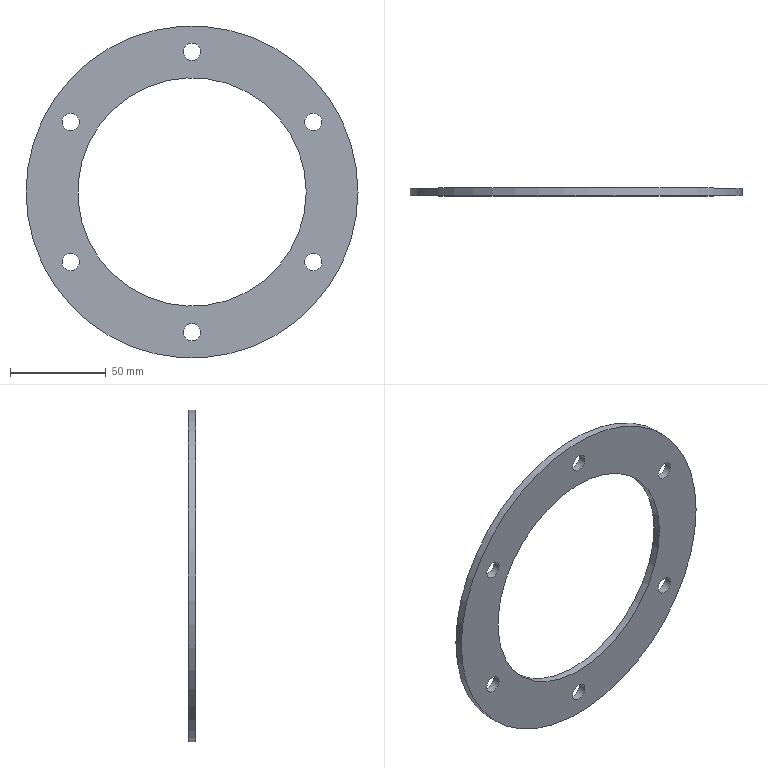Part | NX | features DATUM_CSYS 2, EXTRUDE 1, SKETCH 1 | 1 solid | 10 faces | box 173 x 4 x 173 mm | volume 48010 mm3 | cylinder 8 | plane 2 | commonest cylinder face diameters 9 x6 119 x1 173 x1
STEP:
#1=CARTESIAN_POINT('',(4.5,-4.,73.));
#2=VERTEX_POINT('',#1);
#3=CARTESIAN_POINT('',(0.,-4.,73.));
#4=DIRECTION('',(0.,-1.,0.));
#5=DIRECTION('',(1.,0.,0.));
#6=AXIS2_PLACEMENT_3D('',#3,#4,#5);
#7=CIRCLE('',#6,4.5);
#8=EDGE_CURVE('',#2,#2,#7,.T.);
#9=ORIENTED_EDGE('',*,*,#8,.T.);
#10=EDGE_LOOP('',(#9));
#11=FACE_BOUND('',#10,.T.);
#12=CARTESIAN_POINT('',(4.5,0.,73.));
#13=VERTEX_POINT('',#12);
#14=CARTESIAN_POINT('',(0.,0.,73.));
#15=DIRECTION('',(0.,-1.,0.));
#16=DIRECTION('',(1.,0.,0.));
#17=AXIS2_PLACEMENT_3D('',#14,#15,#16);
#18=CIRCLE('',#17,4.5);
#19=EDGE_CURVE('',#13,#13,#18,.T.);
#20=ORIENTED_EDGE('',*,*,#19,.F.);
#21=EDGE_LOOP('',(#20));
#22=FACE_BOUND('',#21,.T.);
#23=CARTESIAN_POINT('',(0.,-4.,73.));
#24=DIRECTION('',(0.,1.,0.));
#25=DIRECTION('',(0.,0.,1.));
#26=AXIS2_PLACEMENT_3D('',#23,#24,#25);
#27=CYLINDRICAL_SURFACE('',#26,4.5);
#28=ADVANCED_FACE('',(#11,#22),#27,.F.);
#29=CARTESIAN_POINT('',(59.5,-4.,0.));
#30=VERTEX_POINT('',#29);
#31=CARTESIAN_POINT('',(0.,-4.,0.));
#32=DIRECTION('',(0.,-1.,0.));
#33=DIRECTION('',(1.,0.,0.));
#34=AXIS2_PLACEMENT_3D('',#31,#32,#33);
#35=CIRCLE('',#34,59.5);
#36=EDGE_CURVE('',#30,#30,#35,.T.);
#37=ORIENTED_EDGE('',*,*,#36,.T.);
#38=EDGE_LOOP('',(#37));
#39=FACE_BOUND('',#38,.T.);
#40=CARTESIAN_POINT('',(59.5,0.,0.));
#41=VERTEX_POINT('',#40);
#42=CARTESIAN_POINT('',(0.,0.,0.));
#43=DIRECTION('',(0.,-1.,0.));
#44=DIRECTION('',(1.,0.,0.));
#45=AXIS2_PLACEMENT_3D('',#42,#43,#44);
#46=CIRCLE('',#45,59.5);
#47=EDGE_CURVE('',#41,#41,#46,.T.);
#48=ORIENTED_EDGE('',*,*,#47,.F.);
#49=EDGE_LOOP('',(#48));
#50=FACE_BOUND('',#49,.T.);
#51=CARTESIAN_POINT('',(0.,-4.,0.));
#52=DIRECTION('',(0.,1.,0.));
#53=DIRECTION('',(0.,0.,1.));
#54=AXIS2_PLACEMENT_3D('',#51,#52,#53);
#55=CYLINDRICAL_SURFACE('',#54,59.5);
#56=ADVANCED_FACE('',(#39,#50),#55,.F.);
#57=CARTESIAN_POINT('',(-65.47,-4.,-32.603));
#58=VERTEX_POINT('',#57);
#59=CARTESIAN_POINT('',(-63.22,-4.,-36.5));
#60=DIRECTION('',(0.,-1.,0.));
#61=DIRECTION('',(-0.5,0.,0.866));
#62=AXIS2_PLACEMENT_3D('',#59,#60,#61);
#63=CIRCLE('',#62,4.5);
#64=EDGE_CURVE('',#58,#58,#63,.T.);
#65=ORIENTED_EDGE('',*,*,#64,.T.);
#66=EDGE_LOOP('',(#65));
#67=FACE_BOUND('',#66,.T.);
#68=CARTESIAN_POINT('',(-65.47,0.,-32.603));
#69=VERTEX_POINT('',#68);
#70=CARTESIAN_POINT('',(-63.22,0.,-36.5));
#71=DIRECTION('',(0.,-1.,0.));
#72=DIRECTION('',(-0.5,0.,0.866));
#73=AXIS2_PLACEMENT_3D('',#70,#71,#72);
#74=CIRCLE('',#73,4.5);
#75=EDGE_CURVE('',#69,#69,#74,.T.);
#76=ORIENTED_EDGE('',*,*,#75,.F.);
#77=EDGE_LOOP('',(#76));
#78=FACE_BOUND('',#77,.T.);
#79=CARTESIAN_POINT('',(-63.22,-4.,-36.5));
#80=DIRECTION('',(0.,1.,0.));
#81=DIRECTION('',(0.,0.,1.));
#82=AXIS2_PLACEMENT_3D('',#79,#80,#81);
#83=CYLINDRICAL_SURFACE('',#82,4.5);
#84=ADVANCED_FACE('',(#67,#78),#83,.F.);
#85=CARTESIAN_POINT('',(-60.97,-4.,40.397));
#86=VERTEX_POINT('',#85);
#87=CARTESIAN_POINT('',(-63.22,-4.,36.5));
#88=DIRECTION('',(0.,-1.,0.));
#89=DIRECTION('',(0.5,0.,0.866));
#90=AXIS2_PLACEMENT_3D('',#87,#88,#89);
#91=CIRCLE('',#90,4.5);
#92=EDGE_CURVE('',#86,#86,#91,.T.);
#93=ORIENTED_EDGE('',*,*,#92,.T.);
#94=EDGE_LOOP('',(#93));
#95=FACE_BOUND('',#94,.T.);
#96=CARTESIAN_POINT('',(-60.97,0.,40.397));
#97=VERTEX_POINT('',#96);
#98=CARTESIAN_POINT('',(-63.22,0.,36.5));
#99=DIRECTION('',(0.,-1.,0.));
#100=DIRECTION('',(0.5,0.,0.866));
#101=AXIS2_PLACEMENT_3D('',#98,#99,#100);
#102=CIRCLE('',#101,4.5);
#103=EDGE_CURVE('',#97,#97,#102,.T.);
#104=ORIENTED_EDGE('',*,*,#103,.F.);
#105=EDGE_LOOP('',(#104));
#106=FACE_BOUND('',#105,.T.);
#107=CARTESIAN_POINT('',(-63.22,-4.,36.5));
#108=DIRECTION('',(0.,1.,0.));
#109=DIRECTION('',(0.,0.,1.));
#110=AXIS2_PLACEMENT_3D('',#107,#108,#109);
#111=CYLINDRICAL_SURFACE('',#110,4.5);
#112=ADVANCED_FACE('',(#95,#106),#111,.F.);
#113=CARTESIAN_POINT('',(-4.5,-4.,-73.));
#114=VERTEX_POINT('',#113);
#115=CARTESIAN_POINT('',(0.,-4.,-73.));
#116=DIRECTION('',(0.,-1.,0.));
#117=DIRECTION('',(-1.,0.,0.));
#118=AXIS2_PLACEMENT_3D('',#115,#116,#117);
#119=CIRCLE('',#118,4.5);
#120=EDGE_CURVE('',#114,#114,#119,.T.);
#121=ORIENTED_EDGE('',*,*,#120,.T.);
#122=EDGE_LOOP('',(#121));
#123=FACE_BOUND('',#122,.T.);
#124=CARTESIAN_POINT('',(-4.5,0.,-73.));
#125=VERTEX_POINT('',#124);
#126=CARTESIAN_POINT('',(0.,0.,-73.));
#127=DIRECTION('',(0.,-1.,0.));
#128=DIRECTION('',(-1.,0.,0.));
#129=AXIS2_PLACEMENT_3D('',#126,#127,#128);
#130=CIRCLE('',#129,4.5);
#131=EDGE_CURVE('',#125,#125,#130,.T.);
#132=ORIENTED_EDGE('',*,*,#131,.F.);
#133=EDGE_LOOP('',(#132));
#134=FACE_BOUND('',#133,.T.);
#135=CARTESIAN_POINT('',(0.,-4.,-73.));
#136=DIRECTION('',(0.,1.,0.));
#137=DIRECTION('',(0.,0.,1.));
#138=AXIS2_PLACEMENT_3D('',#135,#136,#137);
#139=CYLINDRICAL_SURFACE('',#138,4.5);
#140=ADVANCED_FACE('',(#123,#134),#139,.F.);
#141=CARTESIAN_POINT('',(60.97,-4.,-40.397));
#142=VERTEX_POINT('',#141);
#143=CARTESIAN_POINT('',(63.22,-4.,-36.5));
#144=DIRECTION('',(0.,-1.,0.));
#145=DIRECTION('',(-0.5,0.,-0.866));
#146=AXIS2_PLACEMENT_3D('',#143,#144,#145);
#147=CIRCLE('',#146,4.5);
#148=EDGE_CURVE('',#142,#142,#147,.T.);
#149=ORIENTED_EDGE('',*,*,#148,.T.);
#150=EDGE_LOOP('',(#149));
#151=FACE_BOUND('',#150,.T.);
#152=CARTESIAN_POINT('',(60.97,0.,-40.397));
#153=VERTEX_POINT('',#152);
#154=CARTESIAN_POINT('',(63.22,0.,-36.5));
#155=DIRECTION('',(0.,-1.,0.));
#156=DIRECTION('',(-0.5,0.,-0.866));
#157=AXIS2_PLACEMENT_3D('',#154,#155,#156);
#158=CIRCLE('',#157,4.5);
#159=EDGE_CURVE('',#153,#153,#158,.T.);
#160=ORIENTED_EDGE('',*,*,#159,.F.);
#161=EDGE_LOOP('',(#160));
#162=FACE_BOUND('',#161,.T.);
#163=CARTESIAN_POINT('',(63.22,-4.,-36.5));
#164=DIRECTION('',(0.,1.,0.));
#165=DIRECTION('',(0.,0.,1.));
#166=AXIS2_PLACEMENT_3D('',#163,#164,#165);
#167=CYLINDRICAL_SURFACE('',#166,4.5);
#168=ADVANCED_FACE('',(#151,#162),#167,.F.);
#169=CARTESIAN_POINT('',(86.5,-4.,0.));
#170=VERTEX_POINT('',#169);
#171=CARTESIAN_POINT('',(0.,-4.,0.));
#172=DIRECTION('',(0.,-1.,0.));
#173=DIRECTION('',(1.,0.,0.));
#174=AXIS2_PLACEMENT_3D('',#171,#172,#173);
#175=CIRCLE('',#174,86.5);
#176=EDGE_CURVE('',#170,#170,#175,.T.);
#177=ORIENTED_EDGE('',*,*,#176,.F.);
#178=EDGE_LOOP('',(#177));
#179=FACE_BOUND('',#178,.T.);
#180=CARTESIAN_POINT('',(86.5,0.,0.));
#181=VERTEX_POINT('',#180);
#182=CARTESIAN_POINT('',(0.,0.,0.));
#183=DIRECTION('',(0.,-1.,0.));
#184=DIRECTION('',(1.,0.,0.));
#185=AXIS2_PLACEMENT_3D('',#182,#183,#184);
#186=CIRCLE('',#185,86.5);
#187=EDGE_CURVE('',#181,#181,#186,.T.);
#188=ORIENTED_EDGE('',*,*,#187,.T.);
#189=EDGE_LOOP('',(#188));
#190=FACE_BOUND('',#189,.T.);
#191=CARTESIAN_POINT('',(0.,-4.,0.));
#192=DIRECTION('',(0.,1.,0.));
#193=DIRECTION('',(0.,0.,1.));
#194=AXIS2_PLACEMENT_3D('',#191,#192,#193);
#195=CYLINDRICAL_SURFACE('',#194,86.5);
#196=ADVANCED_FACE('',(#179,#190),#195,.T.);
#197=CARTESIAN_POINT('',(65.47,-4.,32.603));
#198=VERTEX_POINT('',#197);
#199=CARTESIAN_POINT('',(63.22,-4.,36.5));
#200=DIRECTION('',(0.,-1.,0.));
#201=DIRECTION('',(0.5,0.,-0.866));
#202=AXIS2_PLACEMENT_3D('',#199,#200,#201);
#203=CIRCLE('',#202,4.5);
#204=EDGE_CURVE('',#198,#198,#203,.T.);
#205=ORIENTED_EDGE('',*,*,#204,.T.);
#206=EDGE_LOOP('',(#205));
#207=FACE_BOUND('',#206,.T.);
#208=CARTESIAN_POINT('',(65.47,0.,32.603));
#209=VERTEX_POINT('',#208);
#210=CARTESIAN_POINT('',(63.22,0.,36.5));
#211=DIRECTION('',(0.,-1.,0.));
#212=DIRECTION('',(0.5,0.,-0.866));
#213=AXIS2_PLACEMENT_3D('',#210,#211,#212);
#214=CIRCLE('',#213,4.5);
#215=EDGE_CURVE('',#209,#209,#214,.T.);
#216=ORIENTED_EDGE('',*,*,#215,.F.);
#217=EDGE_LOOP('',(#216));
#218=FACE_BOUND('',#217,.T.);
#219=CARTESIAN_POINT('',(63.22,-4.,36.5));
#220=DIRECTION('',(0.,1.,0.));
#221=DIRECTION('',(0.,0.,1.));
#222=AXIS2_PLACEMENT_3D('',#219,#220,#221);
#223=CYLINDRICAL_SURFACE('',#222,4.5);
#224=ADVANCED_FACE('',(#207,#218),#223,.F.);
#225=ORIENTED_EDGE('',*,*,#176,.T.);
#226=EDGE_LOOP('',(#225));
#227=FACE_BOUND('',#226,.T.);
#228=ORIENTED_EDGE('',*,*,#148,.F.);
#229=EDGE_LOOP('',(#228));
#230=FACE_BOUND('',#229,.T.);
#231=ORIENTED_EDGE('',*,*,#120,.F.);
#232=EDGE_LOOP('',(#231));
#233=FACE_BOUND('',#232,.T.);
#234=ORIENTED_EDGE('',*,*,#92,.F.);
#235=EDGE_LOOP('',(#234));
#236=FACE_BOUND('',#235,.T.);
#237=ORIENTED_EDGE('',*,*,#64,.F.);
#238=EDGE_LOOP('',(#237));
#239=FACE_BOUND('',#238,.T.);
#240=ORIENTED_EDGE('',*,*,#36,.F.);
#241=EDGE_LOOP('',(#240));
#242=FACE_BOUND('',#241,.T.);
#243=ORIENTED_EDGE('',*,*,#8,.F.);
#244=EDGE_LOOP('',(#243));
#245=FACE_BOUND('',#244,.T.);
#246=ORIENTED_EDGE('',*,*,#204,.F.);
#247=EDGE_LOOP('',(#246));
#248=FACE_BOUND('',#247,.T.);
#249=CARTESIAN_POINT('',(31.61,-4.,-18.25));
#250=DIRECTION('',(0.,-1.,0.));
#251=DIRECTION('',(0.,0.,-1.));
#252=AXIS2_PLACEMENT_3D('',#249,#250,#251);
#253=PLANE('',#252);
#254=ADVANCED_FACE('',(#227,#230,#233,#236,#239,#242,#245,#248),#253,.T.);
#255=ORIENTED_EDGE('',*,*,#187,.F.);
#256=EDGE_LOOP('',(#255));
#257=FACE_BOUND('',#256,.T.);
#258=ORIENTED_EDGE('',*,*,#159,.T.);
#259=EDGE_LOOP('',(#258));
#260=FACE_BOUND('',#259,.T.);
#261=ORIENTED_EDGE('',*,*,#131,.T.);
#262=EDGE_LOOP('',(#261));
#263=FACE_BOUND('',#262,.T.);
#264=ORIENTED_EDGE('',*,*,#103,.T.);
#265=EDGE_LOOP('',(#264));
#266=FACE_BOUND('',#265,.T.);
#267=ORIENTED_EDGE('',*,*,#75,.T.);
#268=EDGE_LOOP('',(#267));
#269=FACE_BOUND('',#268,.T.);
#270=ORIENTED_EDGE('',*,*,#47,.T.);
#271=EDGE_LOOP('',(#270));
#272=FACE_BOUND('',#271,.T.);
#273=ORIENTED_EDGE('',*,*,#19,.T.);
#274=EDGE_LOOP('',(#273));
#275=FACE_BOUND('',#274,.T.);
#276=ORIENTED_EDGE('',*,*,#215,.T.);
#277=EDGE_LOOP('',(#276));
#278=FACE_BOUND('',#277,.T.);
#279=CARTESIAN_POINT('',(31.61,0.,-18.25));
#280=DIRECTION('',(0.,-1.,0.));
#281=DIRECTION('',(0.,0.,-1.));
#282=AXIS2_PLACEMENT_3D('',#279,#280,#281);
#283=PLANE('',#282);
#284=ADVANCED_FACE('',(#257,#260,#263,#266,#269,#272,#275,#278),#283,.F.);
#285=CLOSED_SHELL('',(#28,#56,#84,#112,#140,#168,#196,#224,#254,#284));
#286=MANIFOLD_SOLID_BREP('',#285);
#287=(LENGTH_UNIT()NAMED_UNIT(*)SI_UNIT(.MILLI.,.METRE.));
#288=UNCERTAINTY_MEASURE_WITH_UNIT(LENGTH_MEASURE(0.00001),#287,'','');
#289=(NAMED_UNIT(*)PLANE_ANGLE_UNIT()SI_UNIT($,.RADIAN.));
#290=(NAMED_UNIT(*)SI_UNIT($,.STERADIAN.)SOLID_ANGLE_UNIT());
#291=(GEOMETRIC_REPRESENTATION_CONTEXT(3)GLOBAL_UNCERTAINTY_ASSIGNED_CONTEXT((#288))GLOBAL_UNIT_ASSIGNED_CONTEXT((#287,#289,#290))REPRESENTATION_CONTEXT('',''));
#292=ADVANCED_BREP_SHAPE_REPRESENTATION('',(#286),#291);